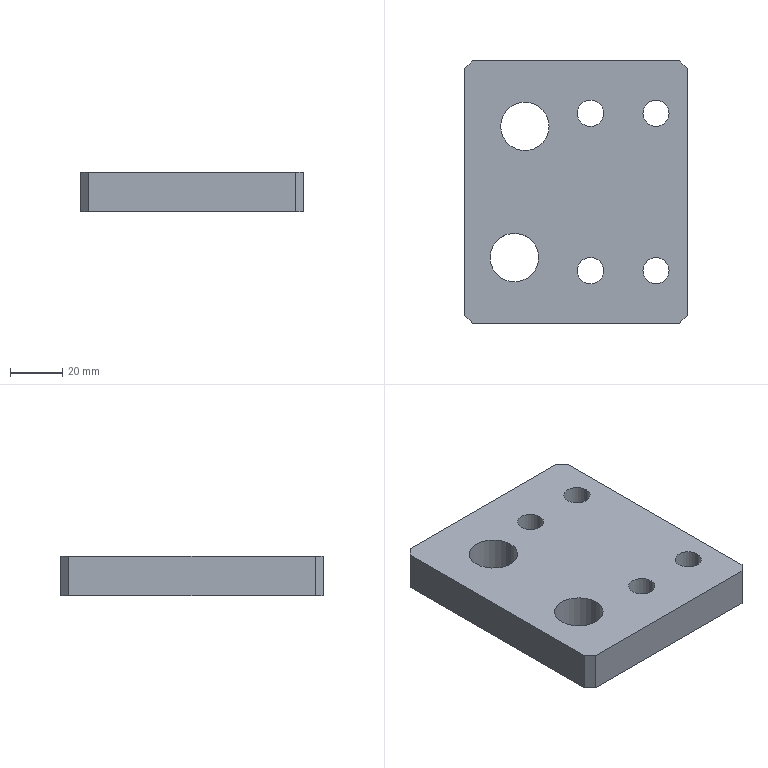Part | STEP file | 1 solid | 22 faces | box 85 x 100 x 15 mm | volume 114454 mm3 | cylinder 12 | plane 10 | commonest cylinder face diameters 10 x8 18.5 x4